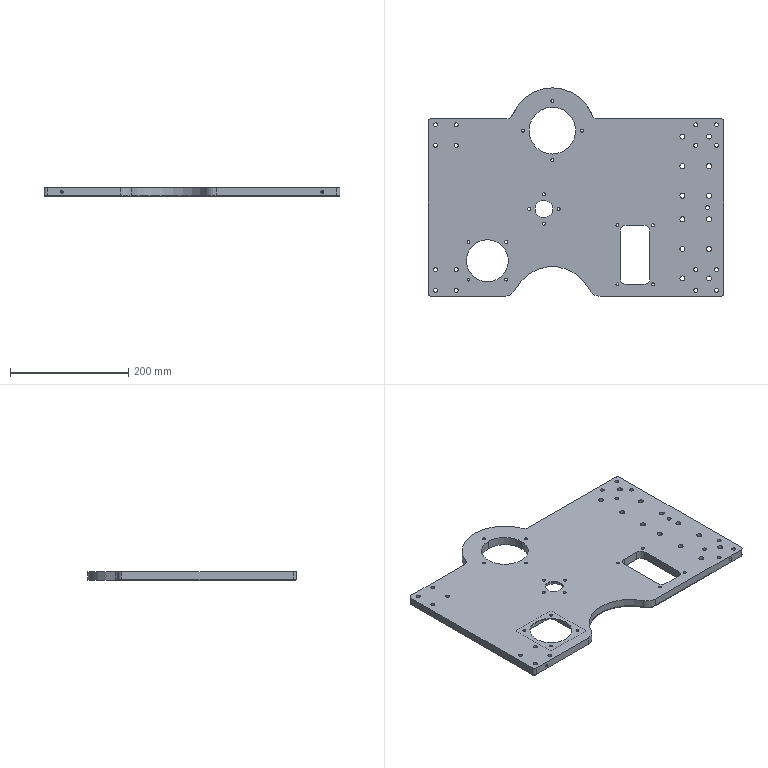CAM job | Mastercam | 3-axis milling, drilling
Tools:
tool_number,name,type,diameter_mm,corner_radius_mm,flutes,flute_length_mm,overall_length_mm,shoulder_length_mm,holder_diameter_mm,length_offset,diameter_offset,default_rpm,default_feed_mm_min,default_plunge_mm_min,coolant
1,5 Drill,drill,5,0,2,25,50,40,50,1,1,1000,75,600,COOL_OFF
2,M6 x 1 RH Tap,drill,6,0,2,24,62,24,50,2,2,200,200,600,COOL_OFF
3,10.5 Drill,drill,10.5,0,2,25,50,40,50,3,3,571,68.52,600,COOL_OFF
4,4 Flat End Mill,end mill,4,0,4,25,75,25,50,4,4,2500,300,600,COOL_OFF
6,6 Flat End Mill,end mill,6,0,4,25,75,25,50,6,6,1667,200.04,600,COOL_OFF
7,4 Chamfer Mill,chamfer mill,4,0,4,25,75,30,50,7,7,6250,750,600,COOL_OFF
8,8 Flat End Mill,end mill,8,0,4,25,75,25,50,8,8,1250,150,600,COOL_OFF
9,8 Bull Nose Mill,bull end mill,8,1,4,25,100,25,50,9,9,1500,180,600,COOL_OFF
9,6.6 Drill,drill,6.6,0,2,25,50,40,50,9,9,909,109.08,600,COOL_OFF
11,8 Bull Nose Mill,bull end mill,8,1,4,25,100,25,50,11,11,1500,180,600,COOL_OFF
14,6.8 Drill,drill,6.8,0,2,25,50,40,50,14,14,882,105.84,600,COOL_OFF
16,16 Flat End Mill,end mill,16,0,4,25,75,25,50,16,16,625,75,600,COOL_OFF
18,8.5 Drill,drill,8.5,0,2,25,50,40,50,18,18,706,84.72,600,COOL_OFF
20,20 Flat End Mill,end mill,20,0,4,25,75,25,50,20,20,500,60,600,COOL_OFF
Operations:
seq,operation,operation_type,tool_number,tool_name,tool_diameter_mm,spindle_rpm,feed_mm_min,plunge_mm_min,retract_mm_min,cycle_time_s,wcs,posted,nc_file
1,Manual Entry (Y direction Clamp plate),ManualEntry,,,,0,0,0,0,0,Plane,yes,.nc
2,Contour (Ramp) - [WCS: Plane] - [Tplane: Plane],Contour,20,20 Flat End Mill,20,5000,4000,600,1200,96.227,Plane,yes,.nc
3,Contour (Ramp) - [WCS: Plane] - [Tplane: Plane],Contour,20,20 Flat End Mill,20,5000,4000,600,1200,60.695,Plane,yes,.nc
4,Contour (Ramp) - [WCS: Plane] - [Tplane: Plane],Contour,20,20 Flat End Mill,20,5000,4000,600,1200,91.417,Plane,yes,.nc
5,Contour (Ramp) - [WCS: Plane] - [Tplane: Plane],Contour,20,20 Flat End Mill,20,5000,3000,600,1200,10.552,Plane,yes,.nc
6,Contour (Ramp) - [WCS: Plane] - [Tplane: Plane],Contour,20,20 Flat End Mill,20,5000,3000,600,1200,15.425,Plane,yes,.nc
7,Contour (Ramp) - [WCS: Plane] - [Tplane: Plane],Contour,20,20 Flat End Mill,20,5000,4000,600,1200,19.085,Plane,yes,.nc
8,Contour (Ramp) - [WCS: Plane] - [Tplane: Plane],Contour,20,20 Flat End Mill,20,5000,4000,600,1200,52.352,Plane,yes,.nc
9,Contour (2D) - [WCS: Plane] - [Tplane: Plane],Contour,16,16 Flat End Mill,16,5000,1000,600,1200,47.43,Plane,yes,.nc
10,Contour (2D) - [WCS: Plane] - [Tplane: Plane],Contour,16,16 Flat End Mill,16,5000,1000,600,1200,13.14,Plane,yes,.nc
11,Contour (2D) - [WCS: Plane] - [Tplane: Plane],Contour,16,16 Flat End Mill,16,5000,1000,600,1200,15.218,Plane,yes,.nc
12,Contour (2D) - [WCS: Plane] - [Tplane: Plane],Contour,16,16 Flat End Mill,16,5000,1000,600,1200,3.903,Plane,yes,.nc
13,Contour (2D) - [WCS: Plane] - [Tplane: Plane],Contour,16,16 Flat End Mill,16,5000,1000,600,1200,5.188,Plane,yes,.nc
14,Contour (2D) - [WCS: Plane] - [Tplane: Plane],Contour,16,16 Flat End Mill,16,5000,1000,600,1200,11.165,Plane,yes,.nc
15,Contour (2D) - [WCS: Plane] - [Tplane: Plane],Contour,16,16 Flat End Mill,16,5000,1000,600,1200,13.069,Plane,yes,.nc
16,2D High Speed (2D Area Mill) - [WCS: Plane] - [Tplane: Plane],HighSpeed2D,8,8 Flat End Mill,8,7000,4000,600,1200,358.632,Plane,yes,.nc
17,Contour (Remachining) - [WCS: Plane] - [Tplane: Plane],Contour,4,4 Flat End Mill,4,6000,3000,600,1200,51.747,Plane,yes,.nc
18,2D High Speed (2D Area Mill) - [WCS: Plane] - [Tplane: Plane],HighSpeed2D,4,4 Flat End Mill,4,6000,1000,600,1200,125.53,Plane,yes,.nc
19,Contour (Ramp) - [WCS: Plane] - [Tplane: Plane],Contour,4,4 Flat End Mill,4,6000,1000,600,1200,111.489,Plane,yes,.nc
20,Drill/Counterbore - [WCS: Plane] - [Tplane: Plane],Drill,7,4 Chamfer Mill,4,6000,200,600,1200,12.851,Plane,yes,.nc
21,Drill/Counterbore - [WCS: Plane] - [Tplane: Plane],Drill,7,4 Chamfer Mill,4,6000,200,600,1200,16.977,Plane,yes,.nc
22,Drill/Counterbore - [WCS: Plane] - [Tplane: Plane],Drill,7,4 Chamfer Mill,4,6000,200,600,1200,11.863,Plane,yes,.nc
23,Peck Drill - [WCS: Plane] - [Tplane: Plane],Drill,18,8.5 Drill,8.5,1000,70,600,1200,172.525,Plane,yes,.nc
24,Peck Drill - [WCS: Plane] - [Tplane: Plane],Drill,14,6.8 Drill,6.8,1000,80,600,1200,12.684,Plane,yes,.nc
25,Peck Drill - [WCS: Plane] - [Tplane: Plane],Drill,1,5 Drill,5,1200,80,600,1200,130.627,Plane,yes,.nc
26,Peck Drill - [WCS: Plane] - [Tplane: Plane],Drill,9,6.6 Drill,6.6,1200,80,600,1200,152.211,Plane,yes,.nc
27,Contour (Ramp) - [WCS: Plane] - [Tplane: Plane],Contour,6,6 Flat End Mill,6,6000,3000,600,1200,62.726,Plane,yes,.nc
28,Contour (Ramp) - [WCS: Plane] - [Tplane: Plane],Contour,6,6 Flat End Mill,6,6000,1000,600,1200,37.446,Plane,yes,.nc
29,Surface Finish Flowline - [WCS: Plane] - [Tplane: Plane],MultiSurfaceFinishFlowline,11,8 Bull Nose Mill,8,6500,4000,600,1200,237.045,Plane,yes,.nc
30,Contour (2D chamfer) - [WCS: Plane] - [Tplane: Plane],Contour,7,4 Chamfer Mill,4,6000,1000,600,1200,98.882,Plane,yes,.nc
31,Contour (2D chamfer) - [WCS: Plane] - [Tplane: Plane],Contour,7,4 Chamfer Mill,4,6000,1000,600,1200,61.76,Plane,yes,.nc
32,Contour (2D chamfer) - [WCS: Plane] - [Tplane: Plane],Contour,7,4 Chamfer Mill,4,6000,1000,600,1200,28.528,Plane,yes,.nc
33,Contour (2D chamfer) - [WCS: Plane] - [Tplane: Plane],Contour,7,4 Chamfer Mill,4,6000,1000,600,1200,21.396,Plane,yes,.nc
34,"Manual Entry (chamfer Clamp plate , move red ， blue 不动)",ManualEntry,,,,0,0,0,0,0,Plane,yes,.nc
35,Manual Entry (M00),ManualEntry,,,,0,0,0,0,0,Plane,yes,.nc
36,Contour (Ramp) - [WCS: Plane] - [Tplane: Plane],Contour,20,20 Flat End Mill,20,5000,4000,600,1200,288.966,Plane,yes,.nc
37,Contour (2D) - [WCS: Plane] - [Tplane: Plane],Contour,16,16 Flat End Mill,16,5000,1000,600,1200,71.502,Plane,yes,.nc
38,Drill/Counterbore - [WCS: Plane] - [Tplane: Plane],Drill,7,4 Chamfer Mill,4,6000,200,600,1200,3.954,Plane,yes,.nc
39,Peck Drill - [WCS: Plane] - [Tplane: Plane],Drill,9,6.6 Drill,6.6,1200,80,600,1200,50.737,Plane,yes,.nc
40,Contour (Ramp) - [WCS: Plane] - [Tplane: Plane],Contour,6,6 Flat End Mill,6,6000,3000,600,1200,20.617,Plane,yes,.nc
41,Contour (Ramp) - [WCS: Plane] - [Tplane: Plane],Contour,6,6 Flat End Mill,6,6000,1000,600,1200,12.372,Plane,yes,.nc
42,3D High Speed (Waterline) - [WCS: Plane] - [Tplane: Plane],HighSpeed3D,11,8 Bull Nose Mill,8,6000,4000,600,1200,42.507,Plane,yes,.nc
43,3D High Speed (Waterline) - [WCS: Plane] - [Tplane: Plane],HighSpeed3D,11,8 Bull Nose Mill,8,6000,4000,600,1200,65.147,Plane,yes,.nc
44,3D High Speed (Waterline) - [WCS: Plane] - [Tplane: Plane],HighSpeed3D,11,8 Bull Nose Mill,8,6000,4000,600,1200,156.657,Plane,yes,.nc
45,Contour (2D chamfer) - [WCS: Plane] - [Tplane: Plane],Contour,7,4 Chamfer Mill,4,6000,1000,600,1200,23.255,Plane,yes,.nc
46,Contour (2D chamfer) - [WCS: Plane] - [Tplane: Plane],Contour,7,4 Chamfer Mill,4,6000,1000,600,1200,10.173,Plane,yes,.nc
47,Manual Entry (G0G90G54X-380.),ManualEntry,,,,0,0,0,0,0,Plane-1,no,
48,Drill/Counterbore - [WCS: Plane-1] - [Tplane: Plane-1],Drill,7,4 Chamfer Mill,4,3000,300,600,1200,2.069,Plane-1,yes,.nc
49,Manual Entry (G0G90G54X-380.),ManualEntry,,,,0,0,0,0,0,Plane-1,no,
50,Peck Drill - [WCS: Plane-1] - [Tplane: Plane-1],Drill,1,5 Drill,5,1000,75,600,1200,41.616,Plane-1,yes,.nc
51,Manual Entry (G0G90G54X-380.),ManualEntry,,,,0,0,0,0,0,Plane-1,no,
52,Contour (2D chamfer) - [WCS: Plane-1] - [Tplane: Plane-1],Contour,7,4 Chamfer Mill,4,6000,500,600,1200,8.306,Plane-1,yes,.nc
53,Manual Entry (G0G90G54X-380.),ManualEntry,,,,0,0,0,0,0,Plane-1,no,
54,Tap - [WCS: Plane-1] - [Tplane: Plane-1],Drill,2,M6 x 1 RH Tap,6,200,200,600,1200,68.786,Plane-1,no,
55,Manual Entry (G0G90G54X-380.),ManualEntry,,,,0,0,0,0,0,Plane-1,no,
56,Drill/Counterbore - [WCS: Plane-2] - [Tplane: Plane-2],Drill,7,4 Chamfer Mill,4,3000,300,600,1200,1.061,Plane-2,yes,.nc
57,Manual Entry (G0G90G54X-380.),ManualEntry,,,,0,0,0,0,0,Plane-1,no,
58,Peck Drill - [WCS: Plane-2] - [Tplane: Plane-2],Drill,1,5 Drill,5,1000,75,600,1200,41.53,Plane-2,yes,.nc
59,Manual Entry (G0G90G54X-380.),ManualEntry,,,,0,0,0,0,0,Plane-1,no,
60,Contour (2D chamfer) - [WCS: Plane-2] - [Tplane: Plane-2],Contour,7,4 Chamfer Mill,4,6000,500,600,1200,7.298,Plane-2,yes,.nc
61,Manual Entry (G0G90G54X-380.),ManualEntry,,,,0,0,0,0,0,Plane-1,no,
62,Tap - [WCS: Plane-2] - [Tplane: Plane-2],Drill,2,M6 x 1 RH Tap,6,200,200,600,1200,36.782,Plane-2,no,
63,Contour (2D) - [WCS: Plane] - [Tplane: Plane],Contour,7,4 Chamfer Mill,4,6000,500,600,1200,48.308,Plane,yes,.nc
64,Drill/Counterbore - [WCS: Plane] - [Tplane: Plane],Drill,7,4 Chamfer Mill,4,6000,200,600,1200,3.503,Plane,yes,.nc
65,Peck Drill - [WCS: Plane] - [Tplane: Plane],Drill,3,10.5 Drill,10.5,800,80,600,1200,106.524,Plane,yes,.nc
66,Contour (2D chamfer) - [WCS: Plane] - [Tplane: Plane],Contour,7,4 Chamfer Mill,4,6000,1000,600,1200,29.475,Plane,yes,.nc